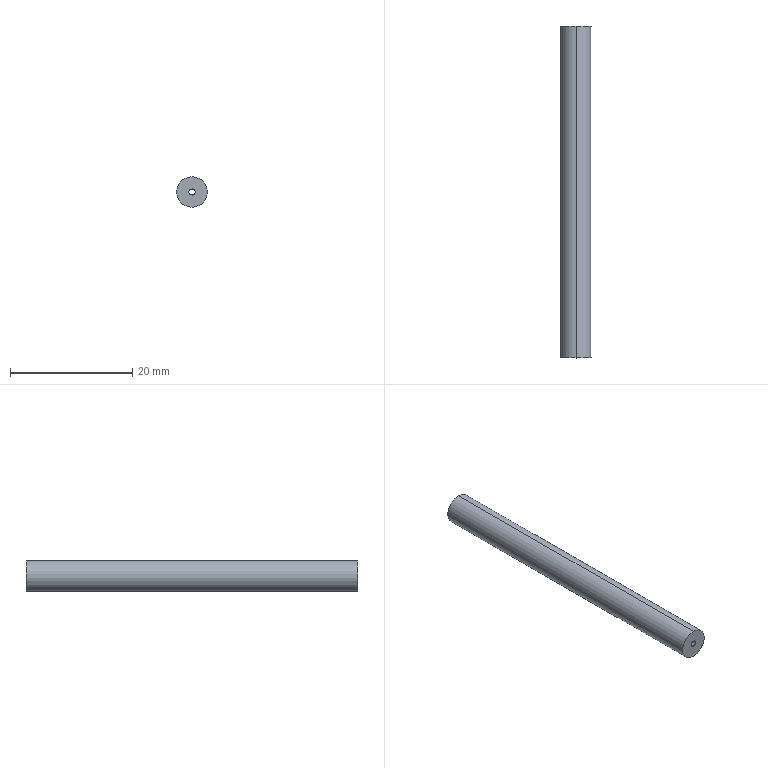Part | SolidWorks | features Extrusion 1, ICE 1 | 1 solid | 9 faces | box 5 x 54.4 x 5 mm | volume 696.177 mm3 | cylinder 6 | plane 3 | commonest cylinder face diameters 1 x2 3 x2 5 x2
STEP:
#1=CARTESIAN_POINT('',(0.,2.,0.5));
#2=VERTEX_POINT('',#1);
#3=CARTESIAN_POINT('',(0.,2.,-0.5));
#4=VERTEX_POINT('',#3);
#5=CARTESIAN_POINT('',(0.,2.,0.));
#6=DIRECTION('',(0.,-1.,0.));
#7=DIRECTION('',(0.,0.,-1.));
#8=AXIS2_PLACEMENT_3D('',#5,#6,#7);
#9=CIRCLE('',#8,0.5);
#10=EDGE_CURVE('',#2,#4,#9,.T.);
#11=ORIENTED_EDGE('',*,*,#10,.F.);
#12=CARTESIAN_POINT('',(0.,0.,0.5));
#13=VERTEX_POINT('',#12);
#14=CARTESIAN_POINT('',(0.,2.,0.5));
#15=DIRECTION('',(0.,-1.,0.));
#16=VECTOR('',#15,1000.);
#17=LINE('',#14,#16);
#18=EDGE_CURVE('',#2,#13,#17,.T.);
#19=ORIENTED_EDGE('',*,*,#18,.T.);
#20=CARTESIAN_POINT('',(0.,0.,-0.5));
#21=VERTEX_POINT('',#20);
#22=CARTESIAN_POINT('',(0.,0.,0.));
#23=DIRECTION('',(0.,-1.,0.));
#24=DIRECTION('',(0.,0.,-1.));
#25=AXIS2_PLACEMENT_3D('',#22,#23,#24);
#26=CIRCLE('',#25,0.5);
#27=EDGE_CURVE('',#13,#21,#26,.T.);
#28=ORIENTED_EDGE('',*,*,#27,.T.);
#29=CARTESIAN_POINT('',(0.,2.,-0.5));
#30=DIRECTION('',(0.,-1.,0.));
#31=VECTOR('',#30,1000.);
#32=LINE('',#29,#31);
#33=EDGE_CURVE('',#4,#21,#32,.T.);
#34=ORIENTED_EDGE('',*,*,#33,.F.);
#35=EDGE_LOOP('',(#11,#19,#28,#34));
#36=FACE_OUTER_BOUND('',#35,.T.);
#37=CARTESIAN_POINT('',(0.,2.,0.));
#38=DIRECTION('',(0.,-1.,0.));
#39=DIRECTION('',(0.,0.,-1.));
#40=AXIS2_PLACEMENT_3D('',#37,#38,#39);
#41=CYLINDRICAL_SURFACE('',#40,0.5);
#42=ADVANCED_FACE('',(#36),#41,.F.);
#43=CARTESIAN_POINT('',(0.,54.4,2.5));
#44=VERTEX_POINT('',#43);
#45=CARTESIAN_POINT('',(0.,54.4,-2.5));
#46=VERTEX_POINT('',#45);
#47=CARTESIAN_POINT('',(0.,54.4,0.));
#48=DIRECTION('',(0.,1.,0.));
#49=DIRECTION('',(0.,0.,1.));
#50=AXIS2_PLACEMENT_3D('',#47,#48,#49);
#51=CIRCLE('',#50,2.5);
#52=EDGE_CURVE('',#44,#46,#51,.T.);
#53=ORIENTED_EDGE('',*,*,#52,.F.);
#54=CARTESIAN_POINT('',(0.,0.,2.5));
#55=VERTEX_POINT('',#54);
#56=CARTESIAN_POINT('',(0.,54.4,2.5));
#57=DIRECTION('',(0.,-1.,0.));
#58=VECTOR('',#57,1000.);
#59=LINE('',#56,#58);
#60=EDGE_CURVE('',#44,#55,#59,.T.);
#61=ORIENTED_EDGE('',*,*,#60,.T.);
#62=CARTESIAN_POINT('',(0.,0.,-2.5));
#63=VERTEX_POINT('',#62);
#64=CARTESIAN_POINT('',(0.,0.,0.));
#65=DIRECTION('',(0.,1.,0.));
#66=DIRECTION('',(0.,0.,1.));
#67=AXIS2_PLACEMENT_3D('',#64,#65,#66);
#68=CIRCLE('',#67,2.5);
#69=EDGE_CURVE('',#55,#63,#68,.T.);
#70=ORIENTED_EDGE('',*,*,#69,.T.);
#71=CARTESIAN_POINT('',(0.,54.4,-2.5));
#72=DIRECTION('',(0.,-1.,0.));
#73=VECTOR('',#72,1000.);
#74=LINE('',#71,#73);
#75=EDGE_CURVE('',#46,#63,#74,.T.);
#76=ORIENTED_EDGE('',*,*,#75,.F.);
#77=EDGE_LOOP('',(#53,#61,#70,#76));
#78=FACE_OUTER_BOUND('',#77,.T.);
#79=CARTESIAN_POINT('',(0.,54.4,0.));
#80=DIRECTION('',(0.,-1.,0.));
#81=DIRECTION('',(0.,0.,-1.));
#82=AXIS2_PLACEMENT_3D('',#79,#80,#81);
#83=CYLINDRICAL_SURFACE('',#82,2.5);
#84=ADVANCED_FACE('',(#78),#83,.T.);
#85=CARTESIAN_POINT('',(0.,54.4,-1.5));
#86=VERTEX_POINT('',#85);
#87=CARTESIAN_POINT('',(0.,54.4,1.5));
#88=VERTEX_POINT('',#87);
#89=CARTESIAN_POINT('',(0.,54.4,0.));
#90=DIRECTION('',(0.,1.,0.));
#91=DIRECTION('',(0.,0.,1.));
#92=AXIS2_PLACEMENT_3D('',#89,#90,#91);
#93=CIRCLE('',#92,1.5);
#94=EDGE_CURVE('',#86,#88,#93,.T.);
#95=ORIENTED_EDGE('',*,*,#94,.T.);
#96=CARTESIAN_POINT('',(0.,2.,1.5));
#97=VERTEX_POINT('',#96);
#98=CARTESIAN_POINT('',(0.,54.4,1.5));
#99=DIRECTION('',(0.,-1.,0.));
#100=VECTOR('',#99,1000.);
#101=LINE('',#98,#100);
#102=EDGE_CURVE('',#88,#97,#101,.T.);
#103=ORIENTED_EDGE('',*,*,#102,.T.);
#104=CARTESIAN_POINT('',(0.,2.,-1.5));
#105=VERTEX_POINT('',#104);
#106=CARTESIAN_POINT('',(0.,2.,0.));
#107=DIRECTION('',(0.,-1.,0.));
#108=DIRECTION('',(0.,0.,-1.));
#109=AXIS2_PLACEMENT_3D('',#106,#107,#108);
#110=CIRCLE('',#109,1.5);
#111=EDGE_CURVE('',#97,#105,#110,.T.);
#112=ORIENTED_EDGE('',*,*,#111,.T.);
#113=CARTESIAN_POINT('',(0.,54.4,-1.5));
#114=DIRECTION('',(0.,-1.,0.));
#115=VECTOR('',#114,1000.);
#116=LINE('',#113,#115);
#117=EDGE_CURVE('',#86,#105,#116,.T.);
#118=ORIENTED_EDGE('',*,*,#117,.F.);
#119=EDGE_LOOP('',(#95,#103,#112,#118));
#120=FACE_OUTER_BOUND('',#119,.T.);
#121=CARTESIAN_POINT('',(0.,54.4,0.));
#122=DIRECTION('',(0.,-1.,0.));
#123=DIRECTION('',(0.,0.,-1.));
#124=AXIS2_PLACEMENT_3D('',#121,#122,#123);
#125=CYLINDRICAL_SURFACE('',#124,1.5);
#126=ADVANCED_FACE('',(#120),#125,.F.);
#127=ORIENTED_EDGE('',*,*,#102,.F.);
#128=CARTESIAN_POINT('',(0.,54.4,0.));
#129=DIRECTION('',(0.,1.,0.));
#130=DIRECTION('',(0.,0.,1.));
#131=AXIS2_PLACEMENT_3D('',#128,#129,#130);
#132=CIRCLE('',#131,1.5);
#133=EDGE_CURVE('',#88,#86,#132,.T.);
#134=ORIENTED_EDGE('',*,*,#133,.T.);
#135=ORIENTED_EDGE('',*,*,#117,.T.);
#136=CARTESIAN_POINT('',(0.,2.,0.));
#137=DIRECTION('',(0.,-1.,0.));
#138=DIRECTION('',(0.,0.,-1.));
#139=AXIS2_PLACEMENT_3D('',#136,#137,#138);
#140=CIRCLE('',#139,1.5);
#141=EDGE_CURVE('',#105,#97,#140,.T.);
#142=ORIENTED_EDGE('',*,*,#141,.T.);
#143=EDGE_LOOP('',(#127,#134,#135,#142));
#144=FACE_OUTER_BOUND('',#143,.T.);
#145=CARTESIAN_POINT('',(0.,54.4,0.));
#146=DIRECTION('',(0.,-1.,0.));
#147=DIRECTION('',(0.,0.,-1.));
#148=AXIS2_PLACEMENT_3D('',#145,#146,#147);
#149=CYLINDRICAL_SURFACE('',#148,1.5);
#150=ADVANCED_FACE('',(#144),#149,.F.);
#151=CARTESIAN_POINT('',(0.,54.4,0.));
#152=DIRECTION('',(0.,1.,0.));
#153=DIRECTION('',(0.,0.,1.));
#154=AXIS2_PLACEMENT_3D('',#151,#152,#153);
#155=CIRCLE('',#154,2.5);
#156=EDGE_CURVE('',#46,#44,#155,.T.);
#157=ORIENTED_EDGE('',*,*,#156,.T.);
#158=ORIENTED_EDGE('',*,*,#52,.T.);
#159=EDGE_LOOP('',(#157,#158));
#160=FACE_OUTER_BOUND('',#159,.T.);
#161=ORIENTED_EDGE('',*,*,#94,.F.);
#162=ORIENTED_EDGE('',*,*,#133,.F.);
#163=EDGE_LOOP('',(#161,#162));
#164=FACE_BOUND('',#163,.T.);
#165=CARTESIAN_POINT('',(0.,54.4,0.));
#166=DIRECTION('',(0.,1.,0.));
#167=DIRECTION('',(0.,0.,1.));
#168=AXIS2_PLACEMENT_3D('',#165,#166,#167);
#169=PLANE('',#168);
#170=ADVANCED_FACE('',(#160,#164),#169,.T.);
#171=CARTESIAN_POINT('',(0.,0.,0.));
#172=DIRECTION('',(0.,1.,0.));
#173=DIRECTION('',(0.,0.,1.));
#174=AXIS2_PLACEMENT_3D('',#171,#172,#173);
#175=CIRCLE('',#174,2.5);
#176=EDGE_CURVE('',#63,#55,#175,.T.);
#177=ORIENTED_EDGE('',*,*,#176,.F.);
#178=ORIENTED_EDGE('',*,*,#69,.F.);
#179=EDGE_LOOP('',(#177,#178));
#180=FACE_OUTER_BOUND('',#179,.T.);
#181=CARTESIAN_POINT('',(0.,0.,0.));
#182=DIRECTION('',(0.,-1.,0.));
#183=DIRECTION('',(0.,0.,-1.));
#184=AXIS2_PLACEMENT_3D('',#181,#182,#183);
#185=CIRCLE('',#184,0.5);
#186=EDGE_CURVE('',#21,#13,#185,.T.);
#187=ORIENTED_EDGE('',*,*,#186,.F.);
#188=ORIENTED_EDGE('',*,*,#27,.F.);
#189=EDGE_LOOP('',(#187,#188));
#190=FACE_BOUND('',#189,.T.);
#191=CARTESIAN_POINT('',(0.,0.,0.));
#192=DIRECTION('',(0.,1.,0.));
#193=DIRECTION('',(0.,0.,1.));
#194=AXIS2_PLACEMENT_3D('',#191,#192,#193);
#195=PLANE('',#194);
#196=ADVANCED_FACE('',(#180,#190),#195,.F.);
#197=ORIENTED_EDGE('',*,*,#60,.F.);
#198=ORIENTED_EDGE('',*,*,#156,.F.);
#199=ORIENTED_EDGE('',*,*,#75,.T.);
#200=ORIENTED_EDGE('',*,*,#176,.T.);
#201=EDGE_LOOP('',(#197,#198,#199,#200));
#202=FACE_OUTER_BOUND('',#201,.T.);
#203=CARTESIAN_POINT('',(0.,54.4,0.));
#204=DIRECTION('',(0.,-1.,0.));
#205=DIRECTION('',(0.,0.,-1.));
#206=AXIS2_PLACEMENT_3D('',#203,#204,#205);
#207=CYLINDRICAL_SURFACE('',#206,2.5);
#208=ADVANCED_FACE('',(#202),#207,.T.);
#209=CARTESIAN_POINT('',(0.,2.,0.));
#210=DIRECTION('',(0.,-1.,0.));
#211=DIRECTION('',(0.,0.,-1.));
#212=AXIS2_PLACEMENT_3D('',#209,#210,#211);
#213=CIRCLE('',#212,0.5);
#214=EDGE_CURVE('',#4,#2,#213,.T.);
#215=ORIENTED_EDGE('',*,*,#214,.T.);
#216=ORIENTED_EDGE('',*,*,#10,.T.);
#217=EDGE_LOOP('',(#215,#216));
#218=FACE_BOUND('',#217,.T.);
#219=ORIENTED_EDGE('',*,*,#141,.F.);
#220=ORIENTED_EDGE('',*,*,#111,.F.);
#221=EDGE_LOOP('',(#219,#220));
#222=FACE_OUTER_BOUND('',#221,.T.);
#223=CARTESIAN_POINT('',(0.,2.,0.));
#224=DIRECTION('',(0.,-1.,0.));
#225=DIRECTION('',(0.,0.,-1.));
#226=AXIS2_PLACEMENT_3D('',#223,#224,#225);
#227=PLANE('',#226);
#228=ADVANCED_FACE('',(#218,#222),#227,.F.);
#229=ORIENTED_EDGE('',*,*,#18,.F.);
#230=ORIENTED_EDGE('',*,*,#214,.F.);
#231=ORIENTED_EDGE('',*,*,#33,.T.);
#232=ORIENTED_EDGE('',*,*,#186,.T.);
#233=EDGE_LOOP('',(#229,#230,#231,#232));
#234=FACE_OUTER_BOUND('',#233,.T.);
#235=CARTESIAN_POINT('',(0.,2.,0.));
#236=DIRECTION('',(0.,-1.,0.));
#237=DIRECTION('',(0.,0.,-1.));
#238=AXIS2_PLACEMENT_3D('',#235,#236,#237);
#239=CYLINDRICAL_SURFACE('',#238,0.5);
#240=ADVANCED_FACE('',(#234),#239,.F.);
#241=CLOSED_SHELL('',(#42,#84,#126,#150,#170,#196,#208,#228,#240));
#242=MANIFOLD_SOLID_BREP('',#241);
#243=CARTESIAN_POINT('',(0.,0.,0.));
#244=DIRECTION('',(0.,0.,1.));
#245=DIRECTION('',(1.,0.,0.));
#246=AXIS2_PLACEMENT_3D('',#243,#244,#245);
#247=(LENGTH_UNIT()NAMED_UNIT(*)SI_UNIT(.MILLI.,.METRE.));
#248=UNCERTAINTY_MEASURE_WITH_UNIT(LENGTH_MEASURE(0.00001),#247,'','');
#249=(NAMED_UNIT(*)PLANE_ANGLE_UNIT()SI_UNIT($,.RADIAN.));
#250=(NAMED_UNIT(*)SI_UNIT($,.STERADIAN.)SOLID_ANGLE_UNIT());
#251=(GEOMETRIC_REPRESENTATION_CONTEXT(3)GLOBAL_UNCERTAINTY_ASSIGNED_CONTEXT((#248))GLOBAL_UNIT_ASSIGNED_CONTEXT((#247,#249,#250))REPRESENTATION_CONTEXT('',''));
#252=ADVANCED_BREP_SHAPE_REPRESENTATION('',(#242,#246),#251);